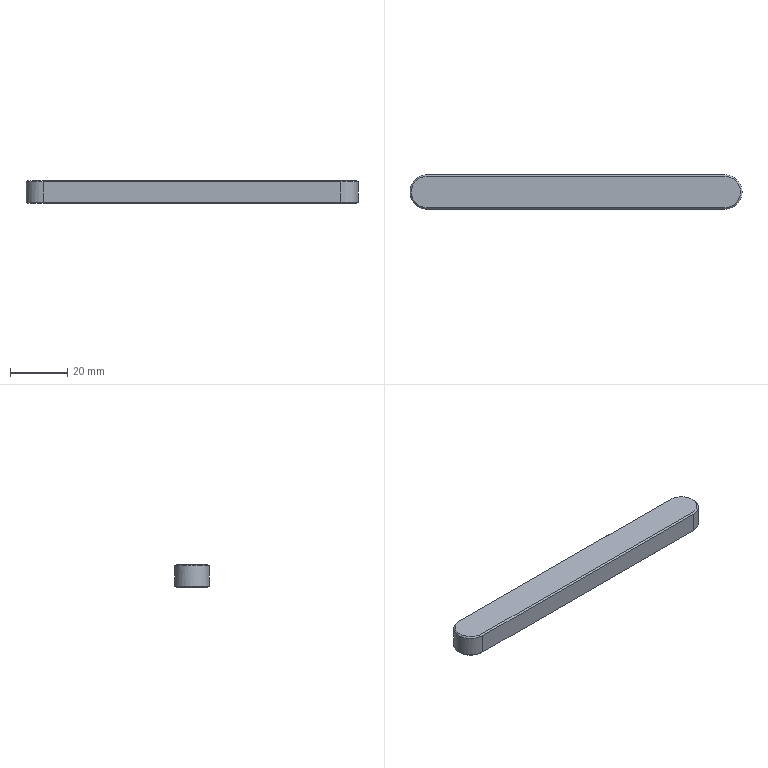Part | SolidWorks | features BaseBody 1 | 1 solid | 17 faces | box 116 x 12 x 8 mm | volume 10828 mm3 | plane 8 | cone 6 | cylinder 3 | commonest cylinder face diameters 12 x3
STEP:
#1=CARTESIAN_POINT('',(71.019,1.374,0.));
#2=VERTEX_POINT('',#1);
#3=CARTESIAN_POINT('',(76.519,6.874,0.));
#4=VERTEX_POINT('',#3);
#5=CARTESIAN_POINT('',(71.019,6.874,0.));
#6=DIRECTION('',(0.,0.,1.));
#7=DIRECTION('',(1.,0.,0.));
#8=AXIS2_PLACEMENT_3D('',#5,#6,#7);
#9=CIRCLE('',#8,5.5);
#10=EDGE_CURVE('',#2,#4,#9,.T.);
#11=ORIENTED_EDGE('',*,*,#10,.T.);
#12=CARTESIAN_POINT('',(77.019,6.874,0.5));
#13=VERTEX_POINT('',#12);
#14=CARTESIAN_POINT('',(77.019,6.874,0.5));
#15=DIRECTION('',(0.7071,0.,0.7071));
#16=VECTOR('',#15,1000.);
#17=LINE('',#14,#16);
#18=EDGE_CURVE('',#4,#13,#17,.T.);
#19=ORIENTED_EDGE('',*,*,#18,.T.);
#20=CARTESIAN_POINT('',(71.019,0.8738,0.5));
#21=VERTEX_POINT('',#20);
#22=CARTESIAN_POINT('',(71.019,6.874,0.5));
#23=DIRECTION('',(0.,0.,-1.));
#24=DIRECTION('',(0.,1.,0.));
#25=AXIS2_PLACEMENT_3D('',#22,#23,#24);
#26=CIRCLE('',#25,6.);
#27=EDGE_CURVE('',#13,#21,#26,.T.);
#28=ORIENTED_EDGE('',*,*,#27,.T.);
#29=CARTESIAN_POINT('',(71.019,1.124,0.25));
#30=DIRECTION('',(0.,-0.7071,0.7071));
#31=VECTOR('',#30,1000.);
#32=LINE('',#29,#31);
#33=EDGE_CURVE('',#2,#21,#32,.T.);
#34=ORIENTED_EDGE('',*,*,#33,.F.);
#35=EDGE_LOOP('',(#11,#19,#28,#34));
#36=FACE_OUTER_BOUND('',#35,.T.);
#37=CARTESIAN_POINT('',(71.019,6.874,0.5));
#38=DIRECTION('',(0.,0.,1.));
#39=DIRECTION('',(1.,0.,0.));
#40=AXIS2_PLACEMENT_3D('',#37,#38,#39);
#41=CONICAL_SURFACE('',#40,6.,0.7854);
#42=ADVANCED_FACE('',(#36),#41,.T.);
#43=ORIENTED_EDGE('',*,*,#27,.F.);
#44=CARTESIAN_POINT('',(77.019,6.874,7.5));
#45=VERTEX_POINT('',#44);
#46=CARTESIAN_POINT('',(77.019,6.874,0.));
#47=DIRECTION('',(0.,0.,1.));
#48=VECTOR('',#47,1000.);
#49=LINE('',#46,#48);
#50=EDGE_CURVE('',#13,#45,#49,.T.);
#51=ORIENTED_EDGE('',*,*,#50,.T.);
#52=CARTESIAN_POINT('',(71.019,0.8738,7.5));
#53=VERTEX_POINT('',#52);
#54=CARTESIAN_POINT('',(71.019,6.874,7.5));
#55=DIRECTION('',(0.,0.,-1.));
#56=DIRECTION('',(1.,0.,0.));
#57=AXIS2_PLACEMENT_3D('',#54,#55,#56);
#58=CIRCLE('',#57,6.);
#59=EDGE_CURVE('',#45,#53,#58,.T.);
#60=ORIENTED_EDGE('',*,*,#59,.T.);
#61=CARTESIAN_POINT('',(71.019,0.8738,0.));
#62=DIRECTION('',(0.,0.,1.));
#63=VECTOR('',#62,1000.);
#64=LINE('',#61,#63);
#65=EDGE_CURVE('',#21,#53,#64,.T.);
#66=ORIENTED_EDGE('',*,*,#65,.F.);
#67=EDGE_LOOP('',(#43,#51,#60,#66));
#68=FACE_OUTER_BOUND('',#67,.T.);
#69=CARTESIAN_POINT('',(71.019,6.874,0.));
#70=DIRECTION('',(0.,0.,1.));
#71=DIRECTION('',(1.,0.,0.));
#72=AXIS2_PLACEMENT_3D('',#69,#70,#71);
#73=CYLINDRICAL_SURFACE('',#72,6.);
#74=ADVANCED_FACE('',(#68),#73,.T.);
#75=CARTESIAN_POINT('',(-32.981,1.374,8.));
#76=VERTEX_POINT('',#75);
#77=CARTESIAN_POINT('',(-38.481,6.874,8.));
#78=VERTEX_POINT('',#77);
#79=CARTESIAN_POINT('',(-32.981,6.874,8.));
#80=DIRECTION('',(0.,0.,-1.));
#81=DIRECTION('',(-1.,0.,0.));
#82=AXIS2_PLACEMENT_3D('',#79,#80,#81);
#83=CIRCLE('',#82,5.5);
#84=EDGE_CURVE('',#76,#78,#83,.T.);
#85=ORIENTED_EDGE('',*,*,#84,.T.);
#86=CARTESIAN_POINT('',(-38.981,6.874,7.5));
#87=VERTEX_POINT('',#86);
#88=CARTESIAN_POINT('',(-38.981,6.874,7.5));
#89=DIRECTION('',(-0.7071,0.,-0.7071));
#90=VECTOR('',#89,1000.);
#91=LINE('',#88,#90);
#92=EDGE_CURVE('',#78,#87,#91,.T.);
#93=ORIENTED_EDGE('',*,*,#92,.T.);
#94=CARTESIAN_POINT('',(-32.981,0.8738,7.5));
#95=VERTEX_POINT('',#94);
#96=CARTESIAN_POINT('',(-32.981,6.874,7.5));
#97=DIRECTION('',(0.,0.,-1.));
#98=DIRECTION('',(1.,0.,0.));
#99=AXIS2_PLACEMENT_3D('',#96,#97,#98);
#100=CIRCLE('',#99,6.);
#101=EDGE_CURVE('',#95,#87,#100,.T.);
#102=ORIENTED_EDGE('',*,*,#101,.F.);
#103=CARTESIAN_POINT('',(-32.981,1.124,7.75));
#104=DIRECTION('',(0.,-0.7071,-0.7071));
#105=VECTOR('',#104,1000.);
#106=LINE('',#103,#105);
#107=EDGE_CURVE('',#76,#95,#106,.T.);
#108=ORIENTED_EDGE('',*,*,#107,.F.);
#109=EDGE_LOOP('',(#85,#93,#102,#108));
#110=FACE_OUTER_BOUND('',#109,.T.);
#111=CARTESIAN_POINT('',(-32.981,6.874,7.5));
#112=DIRECTION('',(0.,0.,-1.));
#113=DIRECTION('',(-1.,0.,0.));
#114=AXIS2_PLACEMENT_3D('',#111,#112,#113);
#115=CONICAL_SURFACE('',#114,6.,0.7854);
#116=ADVANCED_FACE('',(#110),#115,.T.);
#117=CARTESIAN_POINT('',(-32.981,12.374,0.));
#118=VERTEX_POINT('',#117);
#119=CARTESIAN_POINT('',(-32.981,1.374,0.));
#120=VERTEX_POINT('',#119);
#121=CARTESIAN_POINT('',(-32.981,6.874,0.));
#122=DIRECTION('',(0.,0.,1.));
#123=DIRECTION('',(1.,0.,0.));
#124=AXIS2_PLACEMENT_3D('',#121,#122,#123);
#125=CIRCLE('',#124,5.5);
#126=EDGE_CURVE('',#118,#120,#125,.T.);
#127=ORIENTED_EDGE('',*,*,#126,.F.);
#128=CARTESIAN_POINT('',(71.019,12.374,0.));
#129=VERTEX_POINT('',#128);
#130=CARTESIAN_POINT('',(19.019,12.374,0.));
#131=DIRECTION('',(-1.,0.,0.));
#132=VECTOR('',#131,1000.);
#133=LINE('',#130,#132);
#134=EDGE_CURVE('',#129,#118,#133,.T.);
#135=ORIENTED_EDGE('',*,*,#134,.F.);
#136=CARTESIAN_POINT('',(71.019,6.874,0.));
#137=DIRECTION('',(0.,0.,1.));
#138=DIRECTION('',(1.,0.,0.));
#139=AXIS2_PLACEMENT_3D('',#136,#137,#138);
#140=CIRCLE('',#139,5.5);
#141=EDGE_CURVE('',#4,#129,#140,.T.);
#142=ORIENTED_EDGE('',*,*,#141,.F.);
#143=ORIENTED_EDGE('',*,*,#10,.F.);
#144=CARTESIAN_POINT('',(19.019,1.374,0.));
#145=DIRECTION('',(1.,0.,0.));
#146=VECTOR('',#145,1000.);
#147=LINE('',#144,#146);
#148=EDGE_CURVE('',#120,#2,#147,.T.);
#149=ORIENTED_EDGE('',*,*,#148,.F.);
#150=EDGE_LOOP('',(#127,#135,#142,#143,#149));
#151=FACE_OUTER_BOUND('',#150,.T.);
#152=CARTESIAN_POINT('',(19.019,6.874,0.));
#153=DIRECTION('',(0.,0.,1.));
#154=DIRECTION('',(1.,0.,0.));
#155=AXIS2_PLACEMENT_3D('',#152,#153,#154);
#156=PLANE('',#155);
#157=ADVANCED_FACE('',(#151),#156,.F.);
#158=CARTESIAN_POINT('',(-32.981,0.8738,0.5));
#159=VERTEX_POINT('',#158);
#160=CARTESIAN_POINT('',(-32.981,1.124,0.25));
#161=DIRECTION('',(0.,0.7071,-0.7071));
#162=VECTOR('',#161,1000.);
#163=LINE('',#160,#162);
#164=EDGE_CURVE('',#159,#120,#163,.T.);
#165=ORIENTED_EDGE('',*,*,#164,.T.);
#166=ORIENTED_EDGE('',*,*,#148,.T.);
#167=ORIENTED_EDGE('',*,*,#33,.T.);
#168=CARTESIAN_POINT('',(45.019,0.8738,0.5));
#169=DIRECTION('',(-1.,0.,0.));
#170=VECTOR('',#169,1000.);
#171=LINE('',#168,#170);
#172=EDGE_CURVE('',#21,#159,#171,.T.);
#173=ORIENTED_EDGE('',*,*,#172,.T.);
#174=EDGE_LOOP('',(#165,#166,#167,#173));
#175=FACE_OUTER_BOUND('',#174,.T.);
#176=CARTESIAN_POINT('',(45.019,1.124,0.25));
#177=DIRECTION('',(0.,-0.7071,-0.7071));
#178=DIRECTION('',(0.,0.7071,-0.7071));
#179=AXIS2_PLACEMENT_3D('',#176,#177,#178);
#180=PLANE('',#179);
#181=ADVANCED_FACE('',(#175),#180,.T.);
#182=ORIENTED_EDGE('',*,*,#164,.F.);
#183=CARTESIAN_POINT('',(-32.981,12.874,0.5));
#184=VERTEX_POINT('',#183);
#185=CARTESIAN_POINT('',(-32.981,6.874,0.5));
#186=DIRECTION('',(0.,0.,-1.));
#187=DIRECTION('',(0.,-1.,0.));
#188=AXIS2_PLACEMENT_3D('',#185,#186,#187);
#189=CIRCLE('',#188,6.);
#190=EDGE_CURVE('',#159,#184,#189,.T.);
#191=ORIENTED_EDGE('',*,*,#190,.T.);
#192=CARTESIAN_POINT('',(-32.981,499012.374,499000.));
#193=DIRECTION('',(0.,-0.7071,-0.7071));
#194=VECTOR('',#193,1000.);
#195=LINE('',#192,#194);
#196=EDGE_CURVE('',#184,#118,#195,.T.);
#197=ORIENTED_EDGE('',*,*,#196,.T.);
#198=ORIENTED_EDGE('',*,*,#126,.T.);
#199=EDGE_LOOP('',(#182,#191,#197,#198));
#200=FACE_OUTER_BOUND('',#199,.T.);
#201=CARTESIAN_POINT('',(-32.981,6.874,0.5));
#202=DIRECTION('',(0.,0.,1.));
#203=DIRECTION('',(1.,0.,0.));
#204=AXIS2_PLACEMENT_3D('',#201,#202,#203);
#205=CONICAL_SURFACE('',#204,6.,0.7854);
#206=ADVANCED_FACE('',(#200),#205,.T.);
#207=ORIENTED_EDGE('',*,*,#196,.F.);
#208=CARTESIAN_POINT('',(71.019,12.874,0.5));
#209=VERTEX_POINT('',#208);
#210=CARTESIAN_POINT('',(-6.981,12.874,0.5));
#211=DIRECTION('',(1.,0.,0.));
#212=VECTOR('',#211,1000.);
#213=LINE('',#210,#212);
#214=EDGE_CURVE('',#184,#209,#213,.T.);
#215=ORIENTED_EDGE('',*,*,#214,.T.);
#216=CARTESIAN_POINT('',(71.019,12.624,0.25));
#217=DIRECTION('',(0.,-0.7071,-0.7071));
#218=VECTOR('',#217,1000.);
#219=LINE('',#216,#218);
#220=EDGE_CURVE('',#209,#129,#219,.T.);
#221=ORIENTED_EDGE('',*,*,#220,.T.);
#222=ORIENTED_EDGE('',*,*,#134,.T.);
#223=EDGE_LOOP('',(#207,#215,#221,#222));
#224=FACE_OUTER_BOUND('',#223,.T.);
#225=CARTESIAN_POINT('',(-6.981,12.624,0.25));
#226=DIRECTION('',(0.,0.7071,-0.7071));
#227=DIRECTION('',(0.,0.7071,0.7071));
#228=AXIS2_PLACEMENT_3D('',#225,#226,#227);
#229=PLANE('',#228);
#230=ADVANCED_FACE('',(#224),#229,.T.);
#231=ORIENTED_EDGE('',*,*,#18,.F.);
#232=ORIENTED_EDGE('',*,*,#141,.T.);
#233=ORIENTED_EDGE('',*,*,#220,.F.);
#234=CARTESIAN_POINT('',(71.019,6.874,0.5));
#235=DIRECTION('',(0.,0.,-1.));
#236=DIRECTION('',(0.,1.,0.));
#237=AXIS2_PLACEMENT_3D('',#234,#235,#236);
#238=CIRCLE('',#237,6.);
#239=EDGE_CURVE('',#209,#13,#238,.T.);
#240=ORIENTED_EDGE('',*,*,#239,.T.);
#241=EDGE_LOOP('',(#231,#232,#233,#240));
#242=FACE_OUTER_BOUND('',#241,.T.);
#243=CARTESIAN_POINT('',(71.019,6.874,0.5));
#244=DIRECTION('',(0.,0.,1.));
#245=DIRECTION('',(1.,0.,0.));
#246=AXIS2_PLACEMENT_3D('',#243,#244,#245);
#247=CONICAL_SURFACE('',#246,6.,0.7854);
#248=ADVANCED_FACE('',(#242),#247,.T.);
#249=CARTESIAN_POINT('',(71.019,0.8738,7.5));
#250=DIRECTION('',(-1.,0.,0.));
#251=VECTOR('',#250,1000.);
#252=LINE('',#249,#251);
#253=EDGE_CURVE('',#53,#95,#252,.T.);
#254=ORIENTED_EDGE('',*,*,#253,.T.);
#255=CARTESIAN_POINT('',(-32.981,0.8738,0.));
#256=DIRECTION('',(0.,0.,-1.));
#257=VECTOR('',#256,1000.);
#258=LINE('',#255,#257);
#259=EDGE_CURVE('',#95,#159,#258,.T.);
#260=ORIENTED_EDGE('',*,*,#259,.T.);
#261=ORIENTED_EDGE('',*,*,#172,.F.);
#262=ORIENTED_EDGE('',*,*,#65,.T.);
#263=EDGE_LOOP('',(#254,#260,#261,#262));
#264=FACE_OUTER_BOUND('',#263,.T.);
#265=CARTESIAN_POINT('',(71.019,0.8738,0.));
#266=DIRECTION('',(0.,-1.,0.));
#267=DIRECTION('',(1.,0.,0.));
#268=AXIS2_PLACEMENT_3D('',#265,#266,#267);
#269=PLANE('',#268);
#270=ADVANCED_FACE('',(#264),#269,.T.);
#271=ORIENTED_EDGE('',*,*,#101,.T.);
#272=CARTESIAN_POINT('',(-32.981,12.874,7.5));
#273=VERTEX_POINT('',#272);
#274=CARTESIAN_POINT('',(-32.981,6.874,7.5));
#275=DIRECTION('',(0.,0.,-1.));
#276=DIRECTION('',(1.,0.,0.));
#277=AXIS2_PLACEMENT_3D('',#274,#275,#276);
#278=CIRCLE('',#277,6.);
#279=EDGE_CURVE('',#87,#273,#278,.T.);
#280=ORIENTED_EDGE('',*,*,#279,.T.);
#281=CARTESIAN_POINT('',(-32.981,12.874,0.));
#282=DIRECTION('',(0.,0.,-1.));
#283=VECTOR('',#282,1000.);
#284=LINE('',#281,#283);
#285=EDGE_CURVE('',#273,#184,#284,.T.);
#286=ORIENTED_EDGE('',*,*,#285,.T.);
#287=ORIENTED_EDGE('',*,*,#190,.F.);
#288=ORIENTED_EDGE('',*,*,#259,.F.);
#289=EDGE_LOOP('',(#271,#280,#286,#287,#288));
#290=FACE_OUTER_BOUND('',#289,.T.);
#291=CARTESIAN_POINT('',(-32.981,6.874,0.));
#292=DIRECTION('',(0.,0.,1.));
#293=DIRECTION('',(1.,0.,0.));
#294=AXIS2_PLACEMENT_3D('',#291,#292,#293);
#295=CYLINDRICAL_SURFACE('',#294,6.);
#296=ADVANCED_FACE('',(#290),#295,.T.);
#297=CARTESIAN_POINT('',(71.019,12.874,7.5));
#298=VERTEX_POINT('',#297);
#299=CARTESIAN_POINT('',(-32.981,12.874,7.5));
#300=DIRECTION('',(1.,0.,0.));
#301=VECTOR('',#300,1000.);
#302=LINE('',#299,#301);
#303=EDGE_CURVE('',#273,#298,#302,.T.);
#304=ORIENTED_EDGE('',*,*,#303,.T.);
#305=CARTESIAN_POINT('',(71.019,12.874,0.));
#306=DIRECTION('',(0.,0.,-1.));
#307=VECTOR('',#306,1000.);
#308=LINE('',#305,#307);
#309=EDGE_CURVE('',#298,#209,#308,.T.);
#310=ORIENTED_EDGE('',*,*,#309,.T.);
#311=ORIENTED_EDGE('',*,*,#214,.F.);
#312=ORIENTED_EDGE('',*,*,#285,.F.);
#313=EDGE_LOOP('',(#304,#310,#311,#312));
#314=FACE_OUTER_BOUND('',#313,.T.);
#315=CARTESIAN_POINT('',(-32.981,12.874,0.));
#316=DIRECTION('',(0.,1.,0.));
#317=DIRECTION('',(-1.,0.,0.));
#318=AXIS2_PLACEMENT_3D('',#315,#316,#317);
#319=PLANE('',#318);
#320=ADVANCED_FACE('',(#314),#319,.T.);
#321=ORIENTED_EDGE('',*,*,#50,.F.);
#322=ORIENTED_EDGE('',*,*,#239,.F.);
#323=ORIENTED_EDGE('',*,*,#309,.F.);
#324=CARTESIAN_POINT('',(71.019,6.874,7.5));
#325=DIRECTION('',(0.,0.,-1.));
#326=DIRECTION('',(1.,0.,0.));
#327=AXIS2_PLACEMENT_3D('',#324,#325,#326);
#328=CIRCLE('',#327,6.);
#329=EDGE_CURVE('',#298,#45,#328,.T.);
#330=ORIENTED_EDGE('',*,*,#329,.T.);
#331=EDGE_LOOP('',(#321,#322,#323,#330));
#332=FACE_OUTER_BOUND('',#331,.T.);
#333=CARTESIAN_POINT('',(71.019,6.874,0.));
#334=DIRECTION('',(0.,0.,1.));
#335=DIRECTION('',(1.,0.,0.));
#336=AXIS2_PLACEMENT_3D('',#333,#334,#335);
#337=CYLINDRICAL_SURFACE('',#336,6.);
#338=ADVANCED_FACE('',(#332),#337,.T.);
#339=ORIENTED_EDGE('',*,*,#107,.T.);
#340=ORIENTED_EDGE('',*,*,#253,.F.);
#341=CARTESIAN_POINT('',(71.019,1.374,8.));
#342=VERTEX_POINT('',#341);
#343=CARTESIAN_POINT('',(71.019,1.124,7.75));
#344=DIRECTION('',(0.,0.7071,0.7071));
#345=VECTOR('',#344,1000.);
#346=LINE('',#343,#345);
#347=EDGE_CURVE('',#53,#342,#346,.T.);
#348=ORIENTED_EDGE('',*,*,#347,.T.);
#349=CARTESIAN_POINT('',(45.019,1.374,8.));
#350=DIRECTION('',(-1.,0.,0.));
#351=VECTOR('',#350,1000.);
#352=LINE('',#349,#351);
#353=EDGE_CURVE('',#342,#76,#352,.T.);
#354=ORIENTED_EDGE('',*,*,#353,.T.);
#355=EDGE_LOOP('',(#339,#340,#348,#354));
#356=FACE_OUTER_BOUND('',#355,.T.);
#357=CARTESIAN_POINT('',(45.019,1.124,7.75));
#358=DIRECTION('',(0.,-0.7071,0.7071));
#359=DIRECTION('',(0.,-0.7071,-0.7071));
#360=AXIS2_PLACEMENT_3D('',#357,#358,#359);
#361=PLANE('',#360);
#362=ADVANCED_FACE('',(#356),#361,.T.);
#363=ORIENTED_EDGE('',*,*,#92,.F.);
#364=CARTESIAN_POINT('',(-32.981,12.374,8.));
#365=VERTEX_POINT('',#364);
#366=CARTESIAN_POINT('',(-32.981,6.874,8.));
#367=DIRECTION('',(0.,0.,-1.));
#368=DIRECTION('',(-1.,0.,0.));
#369=AXIS2_PLACEMENT_3D('',#366,#367,#368);
#370=CIRCLE('',#369,5.5);
#371=EDGE_CURVE('',#78,#365,#370,.T.);
#372=ORIENTED_EDGE('',*,*,#371,.T.);
#373=CARTESIAN_POINT('',(-32.981,499013.748,-498993.374));
#374=DIRECTION('',(0.,0.7071,-0.7071));
#375=VECTOR('',#374,1000.);
#376=LINE('',#373,#375);
#377=EDGE_CURVE('',#365,#273,#376,.T.);
#378=ORIENTED_EDGE('',*,*,#377,.T.);
#379=ORIENTED_EDGE('',*,*,#279,.F.);
#380=EDGE_LOOP('',(#363,#372,#378,#379));
#381=FACE_OUTER_BOUND('',#380,.T.);
#382=CARTESIAN_POINT('',(-32.981,6.874,7.5));
#383=DIRECTION('',(0.,0.,-1.));
#384=DIRECTION('',(-1.,0.,0.));
#385=AXIS2_PLACEMENT_3D('',#382,#383,#384);
#386=CONICAL_SURFACE('',#385,6.,0.7854);
#387=ADVANCED_FACE('',(#381),#386,.T.);
#388=ORIENTED_EDGE('',*,*,#377,.F.);
#389=CARTESIAN_POINT('',(71.019,12.374,8.));
#390=VERTEX_POINT('',#389);
#391=CARTESIAN_POINT('',(-6.981,12.374,8.));
#392=DIRECTION('',(1.,0.,0.));
#393=VECTOR('',#392,1000.);
#394=LINE('',#391,#393);
#395=EDGE_CURVE('',#365,#390,#394,.T.);
#396=ORIENTED_EDGE('',*,*,#395,.T.);
#397=CARTESIAN_POINT('',(71.019,12.624,7.75));
#398=DIRECTION('',(0.,0.7071,-0.7071));
#399=VECTOR('',#398,1000.);
#400=LINE('',#397,#399);
#401=EDGE_CURVE('',#390,#298,#400,.T.);
#402=ORIENTED_EDGE('',*,*,#401,.T.);
#403=ORIENTED_EDGE('',*,*,#303,.F.);
#404=EDGE_LOOP('',(#388,#396,#402,#403));
#405=FACE_OUTER_BOUND('',#404,.T.);
#406=CARTESIAN_POINT('',(-6.981,12.624,7.75));
#407=DIRECTION('',(0.,0.7071,0.7071));
#408=DIRECTION('',(0.,-0.7071,0.7071));
#409=AXIS2_PLACEMENT_3D('',#406,#407,#408);
#410=PLANE('',#409);
#411=ADVANCED_FACE('',(#405),#410,.T.);
#412=ORIENTED_EDGE('',*,*,#347,.F.);
#413=ORIENTED_EDGE('',*,*,#59,.F.);
#414=ORIENTED_EDGE('',*,*,#329,.F.);
#415=ORIENTED_EDGE('',*,*,#401,.F.);
#416=CARTESIAN_POINT('',(71.019,6.874,8.));
#417=DIRECTION('',(0.,0.,-1.));
#418=DIRECTION('',(-1.,0.,0.));
#419=AXIS2_PLACEMENT_3D('',#416,#417,#418);
#420=CIRCLE('',#419,5.5);
#421=EDGE_CURVE('',#390,#342,#420,.T.);
#422=ORIENTED_EDGE('',*,*,#421,.T.);
#423=EDGE_LOOP('',(#412,#413,#414,#415,#422));
#424=FACE_OUTER_BOUND('',#423,.T.);
#425=CARTESIAN_POINT('',(71.019,6.874,7.5));
#426=DIRECTION('',(0.,0.,-1.));
#427=DIRECTION('',(-1.,0.,0.));
#428=AXIS2_PLACEMENT_3D('',#425,#426,#427);
#429=CONICAL_SURFACE('',#428,6.,0.7854);
#430=ADVANCED_FACE('',(#424),#429,.T.);
#431=ORIENTED_EDGE('',*,*,#395,.F.);
#432=ORIENTED_EDGE('',*,*,#371,.F.);
#433=ORIENTED_EDGE('',*,*,#84,.F.);
#434=ORIENTED_EDGE('',*,*,#353,.F.);
#435=ORIENTED_EDGE('',*,*,#421,.F.);
#436=EDGE_LOOP('',(#431,#432,#433,#434,#435));
#437=FACE_OUTER_BOUND('',#436,.T.);
#438=CARTESIAN_POINT('',(19.019,6.874,8.));
#439=DIRECTION('',(0.,0.,1.));
#440=DIRECTION('',(1.,0.,0.));
#441=AXIS2_PLACEMENT_3D('',#438,#439,#440);
#442=PLANE('',#441);
#443=ADVANCED_FACE('',(#437),#442,.T.);
#444=CLOSED_SHELL('',(#42,#74,#116,#157,#181,#206,#230,#248,#270,#296,#320,#338,#362,#387,#411,#430,#443));
#445=MANIFOLD_SOLID_BREP('',#444);
#446=CARTESIAN_POINT('',(0.,0.,0.));
#447=DIRECTION('',(0.,0.,1.));
#448=DIRECTION('',(1.,0.,0.));
#449=AXIS2_PLACEMENT_3D('',#446,#447,#448);
#450=(LENGTH_UNIT()NAMED_UNIT(*)SI_UNIT(.MILLI.,.METRE.));
#451=UNCERTAINTY_MEASURE_WITH_UNIT(LENGTH_MEASURE(0.00001),#450,'','');
#452=(NAMED_UNIT(*)PLANE_ANGLE_UNIT()SI_UNIT($,.RADIAN.));
#453=(NAMED_UNIT(*)SI_UNIT($,.STERADIAN.)SOLID_ANGLE_UNIT());
#454=(GEOMETRIC_REPRESENTATION_CONTEXT(3)GLOBAL_UNCERTAINTY_ASSIGNED_CONTEXT((#451))GLOBAL_UNIT_ASSIGNED_CONTEXT((#450,#452,#453))REPRESENTATION_CONTEXT('',''));
#455=ADVANCED_BREP_SHAPE_REPRESENTATION('',(#445,#449),#454);